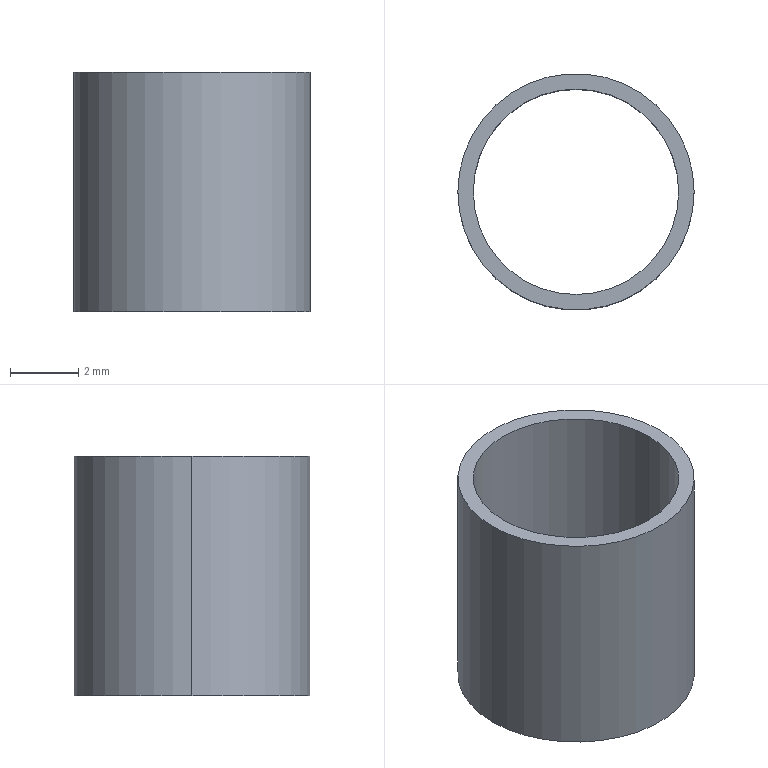Part | SolidWorks | features Extrusion 1 | 1 solid | 6 faces | box 6.9 x 6.9 x 7 mm | volume 63.829 mm3 | cylinder 4 | plane 2 | commonest cylinder face diameters 6 x2 6.9 x2
STEP:
#1=CARTESIAN_POINT('',(-3.,0.,7.));
#2=VERTEX_POINT('',#1);
#3=CARTESIAN_POINT('',(3.,0.,7.));
#4=VERTEX_POINT('',#3);
#5=CARTESIAN_POINT('',(0.,0.,7.));
#6=DIRECTION('',(0.,0.,1.));
#7=DIRECTION('',(1.,0.,0.));
#8=AXIS2_PLACEMENT_3D('',#5,#6,#7);
#9=CIRCLE('',#8,3.);
#10=EDGE_CURVE('',#2,#4,#9,.T.);
#11=ORIENTED_EDGE('',*,*,#10,.T.);
#12=CARTESIAN_POINT('',(3.,0.,0.));
#13=VERTEX_POINT('',#12);
#14=CARTESIAN_POINT('',(3.,0.,7.));
#15=DIRECTION('',(0.,0.,-1.));
#16=VECTOR('',#15,1000.);
#17=LINE('',#14,#16);
#18=EDGE_CURVE('',#4,#13,#17,.T.);
#19=ORIENTED_EDGE('',*,*,#18,.T.);
#20=CARTESIAN_POINT('',(-3.,0.,0.));
#21=VERTEX_POINT('',#20);
#22=CARTESIAN_POINT('',(0.,0.,0.));
#23=DIRECTION('',(0.,0.,1.));
#24=DIRECTION('',(1.,0.,0.));
#25=AXIS2_PLACEMENT_3D('',#22,#23,#24);
#26=CIRCLE('',#25,3.);
#27=EDGE_CURVE('',#21,#13,#26,.T.);
#28=ORIENTED_EDGE('',*,*,#27,.F.);
#29=CARTESIAN_POINT('',(-3.,0.,7.));
#30=DIRECTION('',(0.,0.,-1.));
#31=VECTOR('',#30,1000.);
#32=LINE('',#29,#31);
#33=EDGE_CURVE('',#2,#21,#32,.T.);
#34=ORIENTED_EDGE('',*,*,#33,.F.);
#35=EDGE_LOOP('',(#11,#19,#28,#34));
#36=FACE_OUTER_BOUND('',#35,.T.);
#37=CARTESIAN_POINT('',(0.,0.,7.));
#38=DIRECTION('',(0.,0.,-1.));
#39=DIRECTION('',(-1.,0.,0.));
#40=AXIS2_PLACEMENT_3D('',#37,#38,#39);
#41=CYLINDRICAL_SURFACE('',#40,3.);
#42=ADVANCED_FACE('',(#36),#41,.F.);
#43=CARTESIAN_POINT('',(3.45,0.,7.));
#44=VERTEX_POINT('',#43);
#45=CARTESIAN_POINT('',(-3.45,0.,7.));
#46=VERTEX_POINT('',#45);
#47=CARTESIAN_POINT('',(0.,0.,7.));
#48=DIRECTION('',(0.,0.,1.));
#49=DIRECTION('',(1.,0.,0.));
#50=AXIS2_PLACEMENT_3D('',#47,#48,#49);
#51=CIRCLE('',#50,3.45);
#52=EDGE_CURVE('',#44,#46,#51,.T.);
#53=ORIENTED_EDGE('',*,*,#52,.F.);
#54=CARTESIAN_POINT('',(3.45,0.,0.));
#55=VERTEX_POINT('',#54);
#56=CARTESIAN_POINT('',(3.45,0.,7.));
#57=DIRECTION('',(0.,0.,-1.));
#58=VECTOR('',#57,1000.);
#59=LINE('',#56,#58);
#60=EDGE_CURVE('',#44,#55,#59,.T.);
#61=ORIENTED_EDGE('',*,*,#60,.T.);
#62=CARTESIAN_POINT('',(-3.45,0.,0.));
#63=VERTEX_POINT('',#62);
#64=CARTESIAN_POINT('',(0.,0.,0.));
#65=DIRECTION('',(0.,0.,1.));
#66=DIRECTION('',(1.,0.,0.));
#67=AXIS2_PLACEMENT_3D('',#64,#65,#66);
#68=CIRCLE('',#67,3.45);
#69=EDGE_CURVE('',#55,#63,#68,.T.);
#70=ORIENTED_EDGE('',*,*,#69,.T.);
#71=CARTESIAN_POINT('',(-3.45,0.,7.));
#72=DIRECTION('',(0.,0.,-1.));
#73=VECTOR('',#72,1000.);
#74=LINE('',#71,#73);
#75=EDGE_CURVE('',#46,#63,#74,.T.);
#76=ORIENTED_EDGE('',*,*,#75,.F.);
#77=EDGE_LOOP('',(#53,#61,#70,#76));
#78=FACE_OUTER_BOUND('',#77,.T.);
#79=CARTESIAN_POINT('',(0.,0.,7.));
#80=DIRECTION('',(0.,0.,-1.));
#81=DIRECTION('',(-1.,0.,0.));
#82=AXIS2_PLACEMENT_3D('',#79,#80,#81);
#83=CYLINDRICAL_SURFACE('',#82,3.45);
#84=ADVANCED_FACE('',(#78),#83,.T.);
#85=CARTESIAN_POINT('',(0.,0.,7.));
#86=DIRECTION('',(0.,0.,1.));
#87=DIRECTION('',(1.,0.,0.));
#88=AXIS2_PLACEMENT_3D('',#85,#86,#87);
#89=CIRCLE('',#88,3.45);
#90=EDGE_CURVE('',#46,#44,#89,.T.);
#91=ORIENTED_EDGE('',*,*,#90,.T.);
#92=ORIENTED_EDGE('',*,*,#52,.T.);
#93=EDGE_LOOP('',(#91,#92));
#94=FACE_OUTER_BOUND('',#93,.T.);
#95=ORIENTED_EDGE('',*,*,#10,.F.);
#96=CARTESIAN_POINT('',(0.,0.,7.));
#97=DIRECTION('',(0.,0.,1.));
#98=DIRECTION('',(1.,0.,0.));
#99=AXIS2_PLACEMENT_3D('',#96,#97,#98);
#100=CIRCLE('',#99,3.);
#101=EDGE_CURVE('',#4,#2,#100,.T.);
#102=ORIENTED_EDGE('',*,*,#101,.F.);
#103=EDGE_LOOP('',(#95,#102));
#104=FACE_BOUND('',#103,.T.);
#105=CARTESIAN_POINT('',(0.,0.,7.));
#106=DIRECTION('',(0.,0.,1.));
#107=DIRECTION('',(1.,0.,0.));
#108=AXIS2_PLACEMENT_3D('',#105,#106,#107);
#109=PLANE('',#108);
#110=ADVANCED_FACE('',(#94,#104),#109,.T.);
#111=CARTESIAN_POINT('',(0.,0.,0.));
#112=DIRECTION('',(0.,0.,1.));
#113=DIRECTION('',(1.,0.,0.));
#114=AXIS2_PLACEMENT_3D('',#111,#112,#113);
#115=CIRCLE('',#114,3.45);
#116=EDGE_CURVE('',#63,#55,#115,.T.);
#117=ORIENTED_EDGE('',*,*,#116,.F.);
#118=ORIENTED_EDGE('',*,*,#69,.F.);
#119=EDGE_LOOP('',(#117,#118));
#120=FACE_OUTER_BOUND('',#119,.T.);
#121=ORIENTED_EDGE('',*,*,#27,.T.);
#122=CARTESIAN_POINT('',(0.,0.,0.));
#123=DIRECTION('',(0.,0.,1.));
#124=DIRECTION('',(1.,0.,0.));
#125=AXIS2_PLACEMENT_3D('',#122,#123,#124);
#126=CIRCLE('',#125,3.);
#127=EDGE_CURVE('',#13,#21,#126,.T.);
#128=ORIENTED_EDGE('',*,*,#127,.T.);
#129=EDGE_LOOP('',(#121,#128));
#130=FACE_BOUND('',#129,.T.);
#131=CARTESIAN_POINT('',(0.,0.,0.));
#132=DIRECTION('',(0.,0.,1.));
#133=DIRECTION('',(1.,0.,0.));
#134=AXIS2_PLACEMENT_3D('',#131,#132,#133);
#135=PLANE('',#134);
#136=ADVANCED_FACE('',(#120,#130),#135,.F.);
#137=ORIENTED_EDGE('',*,*,#60,.F.);
#138=ORIENTED_EDGE('',*,*,#90,.F.);
#139=ORIENTED_EDGE('',*,*,#75,.T.);
#140=ORIENTED_EDGE('',*,*,#116,.T.);
#141=EDGE_LOOP('',(#137,#138,#139,#140));
#142=FACE_OUTER_BOUND('',#141,.T.);
#143=CARTESIAN_POINT('',(0.,0.,7.));
#144=DIRECTION('',(0.,0.,-1.));
#145=DIRECTION('',(-1.,0.,0.));
#146=AXIS2_PLACEMENT_3D('',#143,#144,#145);
#147=CYLINDRICAL_SURFACE('',#146,3.45);
#148=ADVANCED_FACE('',(#142),#147,.T.);
#149=ORIENTED_EDGE('',*,*,#18,.F.);
#150=ORIENTED_EDGE('',*,*,#101,.T.);
#151=ORIENTED_EDGE('',*,*,#33,.T.);
#152=ORIENTED_EDGE('',*,*,#127,.F.);
#153=EDGE_LOOP('',(#149,#150,#151,#152));
#154=FACE_OUTER_BOUND('',#153,.T.);
#155=CARTESIAN_POINT('',(0.,0.,7.));
#156=DIRECTION('',(0.,0.,-1.));
#157=DIRECTION('',(-1.,0.,0.));
#158=AXIS2_PLACEMENT_3D('',#155,#156,#157);
#159=CYLINDRICAL_SURFACE('',#158,3.);
#160=ADVANCED_FACE('',(#154),#159,.F.);
#161=CLOSED_SHELL('',(#42,#84,#110,#136,#148,#160));
#162=MANIFOLD_SOLID_BREP('',#161);
#163=CARTESIAN_POINT('',(0.,0.,0.));
#164=DIRECTION('',(0.,0.,1.));
#165=DIRECTION('',(1.,0.,0.));
#166=AXIS2_PLACEMENT_3D('',#163,#164,#165);
#167=(LENGTH_UNIT()NAMED_UNIT(*)SI_UNIT(.MILLI.,.METRE.));
#168=UNCERTAINTY_MEASURE_WITH_UNIT(LENGTH_MEASURE(0.00001),#167,'','');
#169=(NAMED_UNIT(*)PLANE_ANGLE_UNIT()SI_UNIT($,.RADIAN.));
#170=(NAMED_UNIT(*)SI_UNIT($,.STERADIAN.)SOLID_ANGLE_UNIT());
#171=(GEOMETRIC_REPRESENTATION_CONTEXT(3)GLOBAL_UNCERTAINTY_ASSIGNED_CONTEXT((#168))GLOBAL_UNIT_ASSIGNED_CONTEXT((#167,#169,#170))REPRESENTATION_CONTEXT('',''));
#172=ADVANCED_BREP_SHAPE_REPRESENTATION('',(#162,#166),#171);